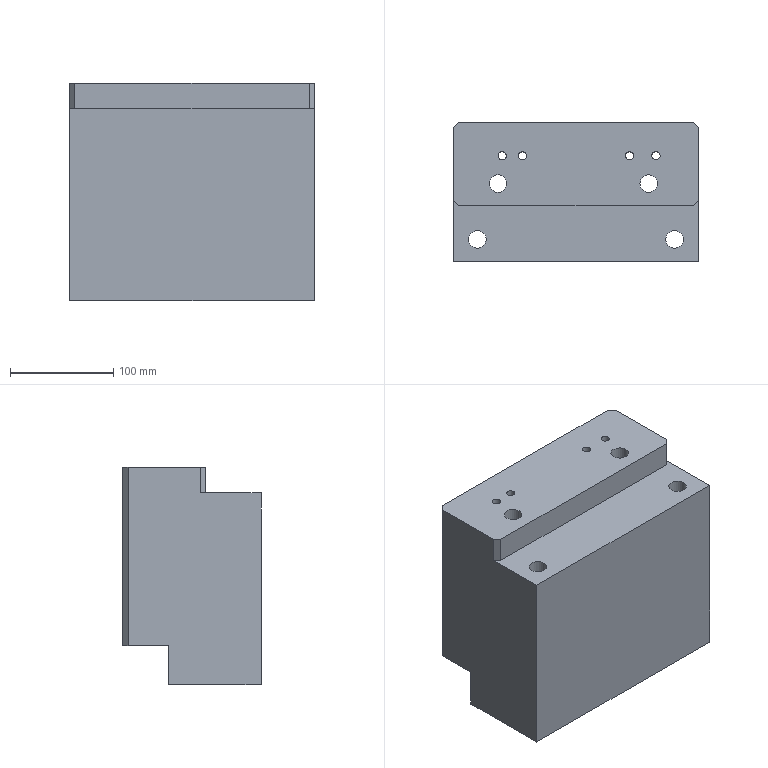Part | NX | features solid 2 | 1 solid | 56 faces | box 237 x 134 x 211 mm | volume 5499408 mm3 | plane 24 | cylinder 19 | cone 10 | spline 3 | commonest cylinder face diameters 8.5 x4 17 x4 26 x4 6 x2 10 x2 10.506 x2